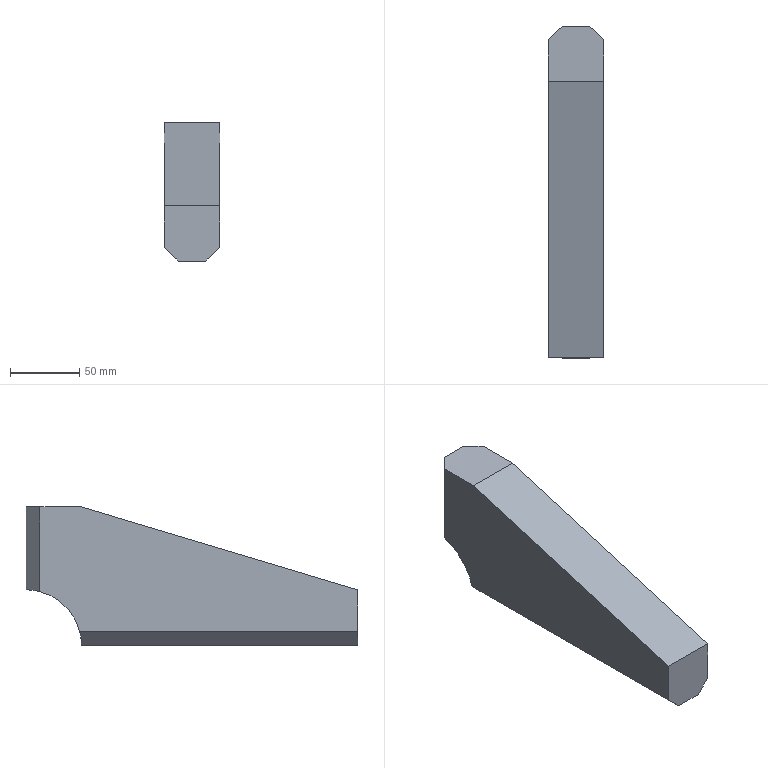Part | SolidWorks | features Chamfer 1, Extrusion 1 | 1 solid | 12 faces | box 40 x 240 x 100 mm | volume 643693 mm3 | plane 11 | cylinder 1 | commonest cylinder face diameters 80 x1
STEP:
#1=CARTESIAN_POINT('',(-20.,0.,40.));
#2=VERTEX_POINT('',#1);
#3=CARTESIAN_POINT('',(-20.,0.,10.));
#4=VERTEX_POINT('',#3);
#5=CARTESIAN_POINT('',(-20.,0.,40.));
#6=DIRECTION('',(0.,0.,-1.));
#7=VECTOR('',#6,1000.);
#8=LINE('',#5,#7);
#9=EDGE_CURVE('',#2,#4,#8,.T.);
#10=ORIENTED_EDGE('',*,*,#9,.T.);
#11=CARTESIAN_POINT('',(-10.,0.,0.));
#12=VERTEX_POINT('',#11);
#13=CARTESIAN_POINT('',(-10.,0.,0.));
#14=DIRECTION('',(0.7071,0.,-0.7071));
#15=VECTOR('',#14,1000.);
#16=LINE('',#13,#15);
#17=EDGE_CURVE('',#4,#12,#16,.T.);
#18=ORIENTED_EDGE('',*,*,#17,.T.);
#19=CARTESIAN_POINT('',(10.,0.,0.));
#20=VERTEX_POINT('',#19);
#21=CARTESIAN_POINT('',(20.,0.,0.));
#22=DIRECTION('',(-1.,0.,0.));
#23=VECTOR('',#22,1000.);
#24=LINE('',#21,#23);
#25=EDGE_CURVE('',#20,#12,#24,.T.);
#26=ORIENTED_EDGE('',*,*,#25,.F.);
#27=CARTESIAN_POINT('',(20.,0.,10.));
#28=VERTEX_POINT('',#27);
#29=CARTESIAN_POINT('',(20.,0.,10.));
#30=DIRECTION('',(0.7071,0.,0.7071));
#31=VECTOR('',#30,1000.);
#32=LINE('',#29,#31);
#33=EDGE_CURVE('',#20,#28,#32,.T.);
#34=ORIENTED_EDGE('',*,*,#33,.T.);
#35=CARTESIAN_POINT('',(20.,0.,40.));
#36=VERTEX_POINT('',#35);
#37=CARTESIAN_POINT('',(20.,0.,40.));
#38=DIRECTION('',(0.,0.,-1.));
#39=VECTOR('',#38,1000.);
#40=LINE('',#37,#39);
#41=EDGE_CURVE('',#36,#28,#40,.T.);
#42=ORIENTED_EDGE('',*,*,#41,.F.);
#43=CARTESIAN_POINT('',(20.,0.,40.));
#44=DIRECTION('',(-1.,0.,0.));
#45=VECTOR('',#44,1000.);
#46=LINE('',#43,#45);
#47=EDGE_CURVE('',#36,#2,#46,.T.);
#48=ORIENTED_EDGE('',*,*,#47,.T.);
#49=EDGE_LOOP('',(#10,#18,#26,#34,#42,#48));
#50=FACE_OUTER_BOUND('',#49,.T.);
#51=CARTESIAN_POINT('',(20.,0.,40.));
#52=DIRECTION('',(0.,1.,0.));
#53=DIRECTION('',(0.,0.,1.));
#54=AXIS2_PLACEMENT_3D('',#51,#52,#53);
#55=PLANE('',#54);
#56=ADVANCED_FACE('',(#50),#55,.F.);
#57=ORIENTED_EDGE('',*,*,#25,.T.);
#58=CARTESIAN_POINT('',(-10.,200.,0.));
#59=VERTEX_POINT('',#58);
#60=CARTESIAN_POINT('',(-10.,0.,0.));
#61=DIRECTION('',(0.,1.,0.));
#62=VECTOR('',#61,1000.);
#63=LINE('',#60,#62);
#64=EDGE_CURVE('',#12,#59,#63,.T.);
#65=ORIENTED_EDGE('',*,*,#64,.T.);
#66=CARTESIAN_POINT('',(10.,200.,0.));
#67=VERTEX_POINT('',#66);
#68=CARTESIAN_POINT('',(20.,200.,0.));
#69=DIRECTION('',(-1.,0.,0.));
#70=VECTOR('',#69,1000.);
#71=LINE('',#68,#70);
#72=EDGE_CURVE('',#67,#59,#71,.T.);
#73=ORIENTED_EDGE('',*,*,#72,.F.);
#74=CARTESIAN_POINT('',(10.,0.,0.));
#75=DIRECTION('',(0.,-1.,0.));
#76=VECTOR('',#75,1000.);
#77=LINE('',#74,#76);
#78=EDGE_CURVE('',#67,#20,#77,.T.);
#79=ORIENTED_EDGE('',*,*,#78,.T.);
#80=EDGE_LOOP('',(#57,#65,#73,#79));
#81=FACE_OUTER_BOUND('',#80,.T.);
#82=CARTESIAN_POINT('',(20.,0.,0.));
#83=DIRECTION('',(0.,0.,1.));
#84=DIRECTION('',(1.,0.,0.));
#85=AXIS2_PLACEMENT_3D('',#82,#83,#84);
#86=PLANE('',#85);
#87=ADVANCED_FACE('',(#81),#86,.F.);
#88=CARTESIAN_POINT('',(10.,240.,40.));
#89=VERTEX_POINT('',#88);
#90=CARTESIAN_POINT('',(-10.,240.,40.));
#91=VERTEX_POINT('',#90);
#92=CARTESIAN_POINT('',(20.,240.,40.));
#93=DIRECTION('',(-1.,0.,0.));
#94=VECTOR('',#93,1000.);
#95=LINE('',#92,#94);
#96=EDGE_CURVE('',#89,#91,#95,.T.);
#97=ORIENTED_EDGE('',*,*,#96,.F.);
#98=CARTESIAN_POINT('',(20.,230.,38.73));
#99=VERTEX_POINT('',#98);
#100=CARTESIAN_POINT('',(10.,240.,40.));
#101=CARTESIAN_POINT('',(13.378,236.622,40.));
#102=CARTESIAN_POINT('',(16.729,233.271,39.574));
#103=CARTESIAN_POINT('',(20.,230.,38.73));
#104=(BOUNDED_CURVE()B_SPLINE_CURVE(3,(#100,#101,#102,#103),.UNSPECIFIED.,.F.,.T.)B_SPLINE_CURVE_WITH_KNOTS((4,4),(1.571,1.823),.UNSPECIFIED.)CURVE()GEOMETRIC_REPRESENTATION_ITEM()RATIONAL_B_SPLINE_CURVE((1.,0.9947,0.9947,1.))REPRESENTATION_ITEM(''));
#105=EDGE_CURVE('',#89,#99,#104,.T.);
#106=ORIENTED_EDGE('',*,*,#105,.T.);
#107=CARTESIAN_POINT('',(20.,201.27,10.));
#108=VERTEX_POINT('',#107);
#109=CARTESIAN_POINT('',(20.,240.,0.));
#110=DIRECTION('',(-1.,0.,0.));
#111=DIRECTION('',(0.,0.,-1.));
#112=AXIS2_PLACEMENT_3D('',#109,#110,#111);
#113=CIRCLE('',#112,40.);
#114=EDGE_CURVE('',#108,#99,#113,.T.);
#115=ORIENTED_EDGE('',*,*,#114,.F.);
#116=CARTESIAN_POINT('',(20.,201.27,10.));
#117=CARTESIAN_POINT('',(16.729,200.426,6.729));
#118=CARTESIAN_POINT('',(13.378,200.,3.378));
#119=CARTESIAN_POINT('',(10.,200.,0.));
#120=(BOUNDED_CURVE()B_SPLINE_CURVE(3,(#116,#117,#118,#119),.UNSPECIFIED.,.F.,.F.)B_SPLINE_CURVE_WITH_KNOTS((4,4),(4.46,4.712),.UNSPECIFIED.)CURVE()GEOMETRIC_REPRESENTATION_ITEM()RATIONAL_B_SPLINE_CURVE((1.,0.9947,0.9947,1.))REPRESENTATION_ITEM(''));
#121=EDGE_CURVE('',#108,#67,#120,.T.);
#122=ORIENTED_EDGE('',*,*,#121,.T.);
#123=ORIENTED_EDGE('',*,*,#72,.T.);
#124=CARTESIAN_POINT('',(-20.,201.27,10.));
#125=VERTEX_POINT('',#124);
#126=CARTESIAN_POINT('',(-10.,200.,0.));
#127=CARTESIAN_POINT('',(-13.378,200.,3.378));
#128=CARTESIAN_POINT('',(-16.729,200.426,6.729));
#129=CARTESIAN_POINT('',(-20.,201.27,10.));
#130=(BOUNDED_CURVE()B_SPLINE_CURVE(3,(#126,#127,#128,#129),.UNSPECIFIED.,.F.,.F.)B_SPLINE_CURVE_WITH_KNOTS((4,4),(4.712,4.965),.UNSPECIFIED.)CURVE()GEOMETRIC_REPRESENTATION_ITEM()RATIONAL_B_SPLINE_CURVE((1.,0.9947,0.9947,1.))REPRESENTATION_ITEM(''));
#131=EDGE_CURVE('',#59,#125,#130,.T.);
#132=ORIENTED_EDGE('',*,*,#131,.T.);
#133=CARTESIAN_POINT('',(-20.,230.,38.73));
#134=VERTEX_POINT('',#133);
#135=CARTESIAN_POINT('',(-20.,240.,0.));
#136=DIRECTION('',(-1.,0.,0.));
#137=DIRECTION('',(0.,0.,-1.));
#138=AXIS2_PLACEMENT_3D('',#135,#136,#137);
#139=CIRCLE('',#138,40.);
#140=EDGE_CURVE('',#125,#134,#139,.T.);
#141=ORIENTED_EDGE('',*,*,#140,.T.);
#142=CARTESIAN_POINT('',(-20.,230.,38.73));
#143=CARTESIAN_POINT('',(-16.729,233.271,39.574));
#144=CARTESIAN_POINT('',(-13.378,236.622,40.));
#145=CARTESIAN_POINT('',(-10.,240.,40.));
#146=(BOUNDED_CURVE()B_SPLINE_CURVE(3,(#142,#143,#144,#145),.UNSPECIFIED.,.F.,.T.)B_SPLINE_CURVE_WITH_KNOTS((4,4),(1.318,1.571),.UNSPECIFIED.)CURVE()GEOMETRIC_REPRESENTATION_ITEM()RATIONAL_B_SPLINE_CURVE((1.,0.9947,0.9947,1.))REPRESENTATION_ITEM(''));
#147=EDGE_CURVE('',#134,#91,#146,.T.);
#148=ORIENTED_EDGE('',*,*,#147,.T.);
#149=EDGE_LOOP('',(#97,#106,#115,#122,#123,#132,#141,#148));
#150=FACE_OUTER_BOUND('',#149,.T.);
#151=CARTESIAN_POINT('',(20.,240.,0.));
#152=DIRECTION('',(-1.,0.,0.));
#153=DIRECTION('',(0.,0.,1.));
#154=AXIS2_PLACEMENT_3D('',#151,#152,#153);
#155=CYLINDRICAL_SURFACE('',#154,40.);
#156=ADVANCED_FACE('',(#150),#155,.F.);
#157=CARTESIAN_POINT('',(10.,240.,100.));
#158=VERTEX_POINT('',#157);
#159=CARTESIAN_POINT('',(-10.,240.,100.));
#160=VERTEX_POINT('',#159);
#161=CARTESIAN_POINT('',(20.,240.,100.));
#162=DIRECTION('',(-1.,0.,0.));
#163=VECTOR('',#162,1000.);
#164=LINE('',#161,#163);
#165=EDGE_CURVE('',#158,#160,#164,.T.);
#166=ORIENTED_EDGE('',*,*,#165,.F.);
#167=CARTESIAN_POINT('',(10.,240.,40.));
#168=DIRECTION('',(0.,0.,-1.));
#169=VECTOR('',#168,1000.);
#170=LINE('',#167,#169);
#171=EDGE_CURVE('',#158,#89,#170,.T.);
#172=ORIENTED_EDGE('',*,*,#171,.T.);
#173=ORIENTED_EDGE('',*,*,#96,.T.);
#174=CARTESIAN_POINT('',(-10.,240.,40.));
#175=DIRECTION('',(0.,0.,1.));
#176=VECTOR('',#175,1000.);
#177=LINE('',#174,#176);
#178=EDGE_CURVE('',#91,#160,#177,.T.);
#179=ORIENTED_EDGE('',*,*,#178,.T.);
#180=EDGE_LOOP('',(#166,#172,#173,#179));
#181=FACE_OUTER_BOUND('',#180,.T.);
#182=CARTESIAN_POINT('',(20.,240.,40.));
#183=DIRECTION('',(0.,-1.,0.));
#184=DIRECTION('',(0.,0.,-1.));
#185=AXIS2_PLACEMENT_3D('',#182,#183,#184);
#186=PLANE('',#185);
#187=ADVANCED_FACE('',(#181),#186,.F.);
#188=CARTESIAN_POINT('',(20.,230.,100.));
#189=VERTEX_POINT('',#188);
#190=CARTESIAN_POINT('',(20.,200.,100.));
#191=VERTEX_POINT('',#190);
#192=CARTESIAN_POINT('',(20.,240.,100.));
#193=DIRECTION('',(0.,-1.,0.));
#194=VECTOR('',#193,1000.);
#195=LINE('',#192,#194);
#196=EDGE_CURVE('',#189,#191,#195,.T.);
#197=ORIENTED_EDGE('',*,*,#196,.F.);
#198=CARTESIAN_POINT('',(20.,230.,100.));
#199=DIRECTION('',(-0.7071,0.7071,0.));
#200=VECTOR('',#199,1000.);
#201=LINE('',#198,#200);
#202=EDGE_CURVE('',#189,#158,#201,.T.);
#203=ORIENTED_EDGE('',*,*,#202,.T.);
#204=ORIENTED_EDGE('',*,*,#165,.T.);
#205=CARTESIAN_POINT('',(-20.,230.,100.));
#206=VERTEX_POINT('',#205);
#207=CARTESIAN_POINT('',(-10.,240.,100.));
#208=DIRECTION('',(-0.7071,-0.7071,0.));
#209=VECTOR('',#208,1000.);
#210=LINE('',#207,#209);
#211=EDGE_CURVE('',#160,#206,#210,.T.);
#212=ORIENTED_EDGE('',*,*,#211,.T.);
#213=CARTESIAN_POINT('',(-20.,200.,100.));
#214=VERTEX_POINT('',#213);
#215=CARTESIAN_POINT('',(-20.,240.,100.));
#216=DIRECTION('',(0.,-1.,0.));
#217=VECTOR('',#216,1000.);
#218=LINE('',#215,#217);
#219=EDGE_CURVE('',#206,#214,#218,.T.);
#220=ORIENTED_EDGE('',*,*,#219,.T.);
#221=CARTESIAN_POINT('',(20.,200.,100.));
#222=DIRECTION('',(-1.,0.,0.));
#223=VECTOR('',#222,1000.);
#224=LINE('',#221,#223);
#225=EDGE_CURVE('',#191,#214,#224,.T.);
#226=ORIENTED_EDGE('',*,*,#225,.F.);
#227=EDGE_LOOP('',(#197,#203,#204,#212,#220,#226));
#228=FACE_OUTER_BOUND('',#227,.T.);
#229=CARTESIAN_POINT('',(20.,240.,100.));
#230=DIRECTION('',(0.,0.,-1.));
#231=DIRECTION('',(-1.,0.,0.));
#232=AXIS2_PLACEMENT_3D('',#229,#230,#231);
#233=PLANE('',#232);
#234=ADVANCED_FACE('',(#228),#233,.F.);
#235=CARTESIAN_POINT('',(-20.,200.,100.));
#236=DIRECTION('',(0.,-0.9578,-0.2873));
#237=VECTOR('',#236,1000.);
#238=LINE('',#235,#237);
#239=EDGE_CURVE('',#214,#2,#238,.T.);
#240=ORIENTED_EDGE('',*,*,#239,.T.);
#241=ORIENTED_EDGE('',*,*,#47,.F.);
#242=CARTESIAN_POINT('',(20.,200.,100.));
#243=DIRECTION('',(0.,-0.9578,-0.2873));
#244=VECTOR('',#243,1000.);
#245=LINE('',#242,#244);
#246=EDGE_CURVE('',#191,#36,#245,.T.);
#247=ORIENTED_EDGE('',*,*,#246,.F.);
#248=ORIENTED_EDGE('',*,*,#225,.T.);
#249=EDGE_LOOP('',(#240,#241,#247,#248));
#250=FACE_OUTER_BOUND('',#249,.T.);
#251=CARTESIAN_POINT('',(20.,200.,100.));
#252=DIRECTION('',(0.,0.2873,-0.9578));
#253=DIRECTION('',(0.,0.9578,0.2873));
#254=AXIS2_PLACEMENT_3D('',#251,#252,#253);
#255=PLANE('',#254);
#256=ADVANCED_FACE('',(#250),#255,.F.);
#257=ORIENTED_EDGE('',*,*,#114,.T.);
#258=CARTESIAN_POINT('',(20.,230.,100.));
#259=DIRECTION('',(0.,0.,1.));
#260=VECTOR('',#259,1000.);
#261=LINE('',#258,#260);
#262=EDGE_CURVE('',#99,#189,#261,.T.);
#263=ORIENTED_EDGE('',*,*,#262,.T.);
#264=ORIENTED_EDGE('',*,*,#196,.T.);
#265=ORIENTED_EDGE('',*,*,#246,.T.);
#266=ORIENTED_EDGE('',*,*,#41,.T.);
#267=CARTESIAN_POINT('',(20.,200.,10.));
#268=DIRECTION('',(0.,1.,0.));
#269=VECTOR('',#268,1000.);
#270=LINE('',#267,#269);
#271=EDGE_CURVE('',#28,#108,#270,.T.);
#272=ORIENTED_EDGE('',*,*,#271,.T.);
#273=EDGE_LOOP('',(#257,#263,#264,#265,#266,#272));
#274=FACE_OUTER_BOUND('',#273,.T.);
#275=CARTESIAN_POINT('',(20.,240.,0.));
#276=DIRECTION('',(1.,0.,0.));
#277=DIRECTION('',(0.,0.,-1.));
#278=AXIS2_PLACEMENT_3D('',#275,#276,#277);
#279=PLANE('',#278);
#280=ADVANCED_FACE('',(#274),#279,.T.);
#281=ORIENTED_EDGE('',*,*,#219,.F.);
#282=CARTESIAN_POINT('',(-20.,230.,0.));
#283=DIRECTION('',(0.,0.,-1.));
#284=VECTOR('',#283,1000.);
#285=LINE('',#282,#284);
#286=EDGE_CURVE('',#206,#134,#285,.T.);
#287=ORIENTED_EDGE('',*,*,#286,.T.);
#288=ORIENTED_EDGE('',*,*,#140,.F.);
#289=CARTESIAN_POINT('',(-20.,240.,10.));
#290=DIRECTION('',(0.,-1.,0.));
#291=VECTOR('',#290,1000.);
#292=LINE('',#289,#291);
#293=EDGE_CURVE('',#125,#4,#292,.T.);
#294=ORIENTED_EDGE('',*,*,#293,.T.);
#295=ORIENTED_EDGE('',*,*,#9,.F.);
#296=ORIENTED_EDGE('',*,*,#239,.F.);
#297=EDGE_LOOP('',(#281,#287,#288,#294,#295,#296));
#298=FACE_OUTER_BOUND('',#297,.T.);
#299=CARTESIAN_POINT('',(-20.,240.,0.));
#300=DIRECTION('',(1.,0.,0.));
#301=DIRECTION('',(0.,0.,-1.));
#302=AXIS2_PLACEMENT_3D('',#299,#300,#301);
#303=PLANE('',#302);
#304=ADVANCED_FACE('',(#298),#303,.F.);
#305=ORIENTED_EDGE('',*,*,#105,.F.);
#306=ORIENTED_EDGE('',*,*,#171,.F.);
#307=ORIENTED_EDGE('',*,*,#202,.F.);
#308=ORIENTED_EDGE('',*,*,#262,.F.);
#309=EDGE_LOOP('',(#305,#306,#307,#308));
#310=FACE_OUTER_BOUND('',#309,.T.);
#311=CARTESIAN_POINT('',(20.,230.,0.));
#312=DIRECTION('',(0.7071,0.7071,0.));
#313=DIRECTION('',(0.,0.,-1.));
#314=AXIS2_PLACEMENT_3D('',#311,#312,#313);
#315=PLANE('',#314);
#316=ADVANCED_FACE('',(#310),#315,.T.);
#317=ORIENTED_EDGE('',*,*,#147,.F.);
#318=ORIENTED_EDGE('',*,*,#286,.F.);
#319=ORIENTED_EDGE('',*,*,#211,.F.);
#320=ORIENTED_EDGE('',*,*,#178,.F.);
#321=EDGE_LOOP('',(#317,#318,#319,#320));
#322=FACE_OUTER_BOUND('',#321,.T.);
#323=CARTESIAN_POINT('',(-10.,240.,40.));
#324=DIRECTION('',(0.7071,-0.7071,0.));
#325=DIRECTION('',(0.,0.,1.));
#326=AXIS2_PLACEMENT_3D('',#323,#324,#325);
#327=PLANE('',#326);
#328=ADVANCED_FACE('',(#322),#327,.F.);
#329=ORIENTED_EDGE('',*,*,#17,.F.);
#330=ORIENTED_EDGE('',*,*,#293,.F.);
#331=ORIENTED_EDGE('',*,*,#131,.F.);
#332=ORIENTED_EDGE('',*,*,#64,.F.);
#333=EDGE_LOOP('',(#329,#330,#331,#332));
#334=FACE_OUTER_BOUND('',#333,.T.);
#335=CARTESIAN_POINT('',(-10.,0.,0.));
#336=DIRECTION('',(0.7071,0.,0.7071));
#337=DIRECTION('',(0.,1.,0.));
#338=AXIS2_PLACEMENT_3D('',#335,#336,#337);
#339=PLANE('',#338);
#340=ADVANCED_FACE('',(#334),#339,.F.);
#341=ORIENTED_EDGE('',*,*,#33,.F.);
#342=ORIENTED_EDGE('',*,*,#78,.F.);
#343=ORIENTED_EDGE('',*,*,#121,.F.);
#344=ORIENTED_EDGE('',*,*,#271,.F.);
#345=EDGE_LOOP('',(#341,#342,#343,#344));
#346=FACE_OUTER_BOUND('',#345,.T.);
#347=CARTESIAN_POINT('',(20.,240.,10.));
#348=DIRECTION('',(0.7071,0.,-0.7071));
#349=DIRECTION('',(0.,-1.,0.));
#350=AXIS2_PLACEMENT_3D('',#347,#348,#349);
#351=PLANE('',#350);
#352=ADVANCED_FACE('',(#346),#351,.T.);
#353=CLOSED_SHELL('',(#56,#87,#156,#187,#234,#256,#280,#304,#316,#328,#340,#352));
#354=MANIFOLD_SOLID_BREP('',#353);
#355=CARTESIAN_POINT('',(0.,0.,0.));
#356=DIRECTION('',(0.,0.,1.));
#357=DIRECTION('',(1.,0.,0.));
#358=AXIS2_PLACEMENT_3D('',#355,#356,#357);
#359=(LENGTH_UNIT()NAMED_UNIT(*)SI_UNIT(.MILLI.,.METRE.));
#360=UNCERTAINTY_MEASURE_WITH_UNIT(LENGTH_MEASURE(0.00001),#359,'','');
#361=(NAMED_UNIT(*)PLANE_ANGLE_UNIT()SI_UNIT($,.RADIAN.));
#362=(NAMED_UNIT(*)SI_UNIT($,.STERADIAN.)SOLID_ANGLE_UNIT());
#363=(GEOMETRIC_REPRESENTATION_CONTEXT(3)GLOBAL_UNCERTAINTY_ASSIGNED_CONTEXT((#360))GLOBAL_UNIT_ASSIGNED_CONTEXT((#359,#361,#362))REPRESENTATION_CONTEXT('',''));
#364=ADVANCED_BREP_SHAPE_REPRESENTATION('',(#354,#358),#363);